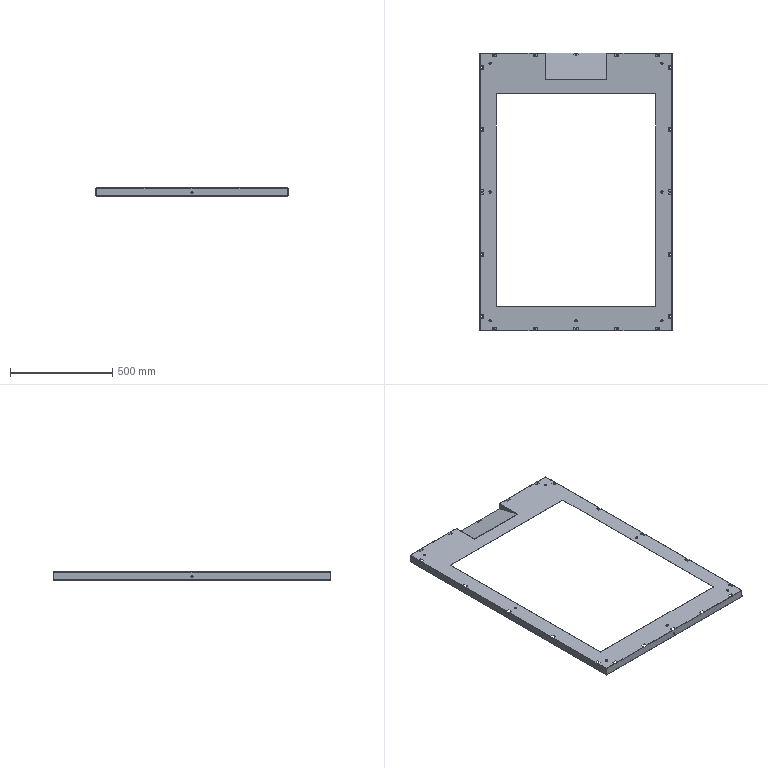Part | SolidWorks | 2 solids | 408 faces | box 939 x 1359 x 40 mm | volume 746249 mm3 | plane 258 | cylinder 130 | spline 20 | commonest cylinder face diameters 7 x50 0.4 x30 2.4 x30 11 x14 10 x6